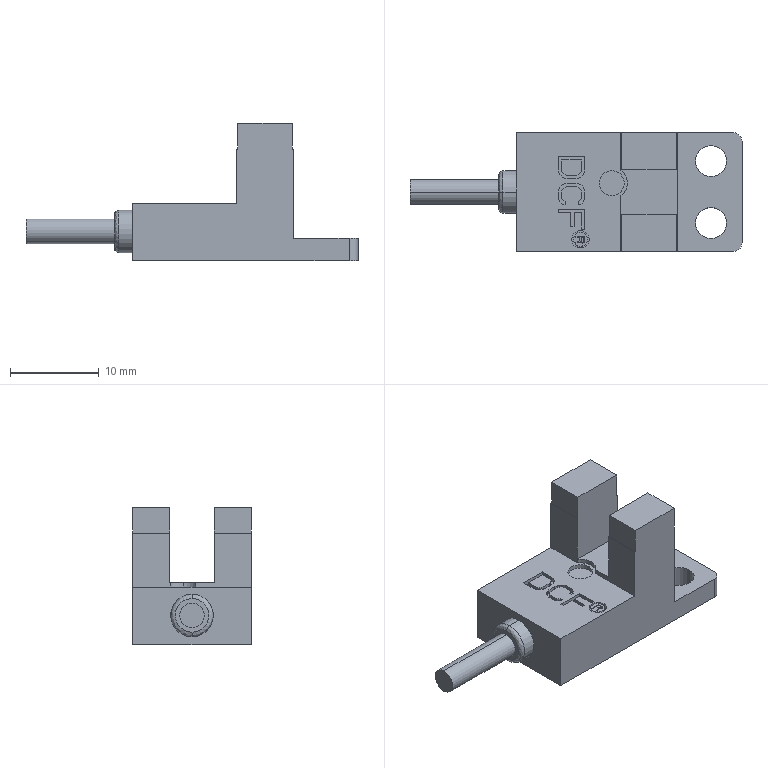Part | SolidWorks | features BaseBody 1 | 1 solid | 156 faces | box 37.5 x 13.4 x 15.5 mm | volume 2365 mm3 | plane 136 | cylinder 18 | spline 2 | commonest cylinder face diameters 3.5 x6 2.8 x4 1.608 x2 1.962 x2 2 x2 4.8 x2